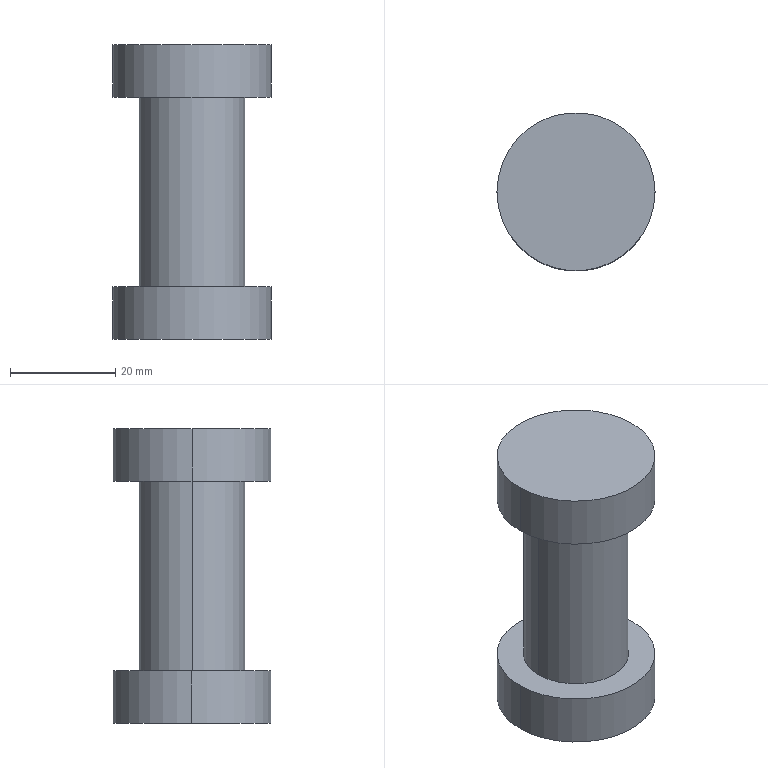Part | SolidWorks | features ICE 2, Extrusion 1 | 1 solid | 10 faces | box 30 x 30 x 56 mm | volume 25447 mm3 | cylinder 6 | plane 4 | commonest cylinder face diameters 30 x4 20 x2
STEP:
#1=CARTESIAN_POINT('',(-15.,0.,-10.));
#2=VERTEX_POINT('',#1);
#3=CARTESIAN_POINT('',(15.,0.,-10.));
#4=VERTEX_POINT('',#3);
#5=CARTESIAN_POINT('',(0.,0.,-10.));
#6=DIRECTION('',(0.,0.,-1.));
#7=DIRECTION('',(-1.,0.,0.));
#8=AXIS2_PLACEMENT_3D('',#5,#6,#7);
#9=CIRCLE('',#8,15.);
#10=EDGE_CURVE('',#2,#4,#9,.T.);
#11=ORIENTED_EDGE('',*,*,#10,.F.);
#12=CARTESIAN_POINT('',(-15.,0.,0.));
#13=VERTEX_POINT('',#12);
#14=CARTESIAN_POINT('',(-15.,0.,-10.));
#15=DIRECTION('',(0.,0.,1.));
#16=VECTOR('',#15,1000.);
#17=LINE('',#14,#16);
#18=EDGE_CURVE('',#2,#13,#17,.T.);
#19=ORIENTED_EDGE('',*,*,#18,.T.);
#20=CARTESIAN_POINT('',(15.,0.,0.));
#21=VERTEX_POINT('',#20);
#22=CARTESIAN_POINT('',(0.,0.,0.));
#23=DIRECTION('',(0.,0.,-1.));
#24=DIRECTION('',(-1.,0.,0.));
#25=AXIS2_PLACEMENT_3D('',#22,#23,#24);
#26=CIRCLE('',#25,15.);
#27=EDGE_CURVE('',#13,#21,#26,.T.);
#28=ORIENTED_EDGE('',*,*,#27,.T.);
#29=CARTESIAN_POINT('',(15.,0.,-10.));
#30=DIRECTION('',(0.,0.,1.));
#31=VECTOR('',#30,1000.);
#32=LINE('',#29,#31);
#33=EDGE_CURVE('',#4,#21,#32,.T.);
#34=ORIENTED_EDGE('',*,*,#33,.F.);
#35=EDGE_LOOP('',(#11,#19,#28,#34));
#36=FACE_OUTER_BOUND('',#35,.T.);
#37=CARTESIAN_POINT('',(0.,0.,-10.));
#38=DIRECTION('',(0.,0.,1.));
#39=DIRECTION('',(1.,0.,0.));
#40=AXIS2_PLACEMENT_3D('',#37,#38,#39);
#41=CYLINDRICAL_SURFACE('',#40,15.);
#42=ADVANCED_FACE('',(#36),#41,.T.);
#43=CARTESIAN_POINT('',(15.,0.,46.));
#44=VERTEX_POINT('',#43);
#45=CARTESIAN_POINT('',(-15.,0.,46.));
#46=VERTEX_POINT('',#45);
#47=CARTESIAN_POINT('',(0.,0.,46.));
#48=DIRECTION('',(0.,0.,1.));
#49=DIRECTION('',(1.,0.,0.));
#50=AXIS2_PLACEMENT_3D('',#47,#48,#49);
#51=CIRCLE('',#50,15.);
#52=EDGE_CURVE('',#44,#46,#51,.T.);
#53=ORIENTED_EDGE('',*,*,#52,.F.);
#54=CARTESIAN_POINT('',(15.,0.,36.));
#55=VERTEX_POINT('',#54);
#56=CARTESIAN_POINT('',(15.,0.,46.));
#57=DIRECTION('',(0.,0.,-1.));
#58=VECTOR('',#57,1000.);
#59=LINE('',#56,#58);
#60=EDGE_CURVE('',#44,#55,#59,.T.);
#61=ORIENTED_EDGE('',*,*,#60,.T.);
#62=CARTESIAN_POINT('',(-15.,0.,36.));
#63=VERTEX_POINT('',#62);
#64=CARTESIAN_POINT('',(0.,0.,36.));
#65=DIRECTION('',(0.,0.,1.));
#66=DIRECTION('',(1.,0.,0.));
#67=AXIS2_PLACEMENT_3D('',#64,#65,#66);
#68=CIRCLE('',#67,15.);
#69=EDGE_CURVE('',#55,#63,#68,.T.);
#70=ORIENTED_EDGE('',*,*,#69,.T.);
#71=CARTESIAN_POINT('',(-15.,0.,46.));
#72=DIRECTION('',(0.,0.,-1.));
#73=VECTOR('',#72,1000.);
#74=LINE('',#71,#73);
#75=EDGE_CURVE('',#46,#63,#74,.T.);
#76=ORIENTED_EDGE('',*,*,#75,.F.);
#77=EDGE_LOOP('',(#53,#61,#70,#76));
#78=FACE_OUTER_BOUND('',#77,.T.);
#79=CARTESIAN_POINT('',(0.,0.,46.));
#80=DIRECTION('',(0.,0.,-1.));
#81=DIRECTION('',(-1.,0.,0.));
#82=AXIS2_PLACEMENT_3D('',#79,#80,#81);
#83=CYLINDRICAL_SURFACE('',#82,15.);
#84=ADVANCED_FACE('',(#78),#83,.T.);
#85=CARTESIAN_POINT('',(10.,0.,36.));
#86=VERTEX_POINT('',#85);
#87=CARTESIAN_POINT('',(-10.,0.,36.));
#88=VERTEX_POINT('',#87);
#89=CARTESIAN_POINT('',(0.,0.,36.));
#90=DIRECTION('',(0.,0.,1.));
#91=DIRECTION('',(1.,0.,0.));
#92=AXIS2_PLACEMENT_3D('',#89,#90,#91);
#93=CIRCLE('',#92,10.);
#94=EDGE_CURVE('',#86,#88,#93,.T.);
#95=ORIENTED_EDGE('',*,*,#94,.F.);
#96=CARTESIAN_POINT('',(10.,0.,0.));
#97=VERTEX_POINT('',#96);
#98=CARTESIAN_POINT('',(10.,0.,36.));
#99=DIRECTION('',(0.,0.,-1.));
#100=VECTOR('',#99,1000.);
#101=LINE('',#98,#100);
#102=EDGE_CURVE('',#86,#97,#101,.T.);
#103=ORIENTED_EDGE('',*,*,#102,.T.);
#104=CARTESIAN_POINT('',(-10.,0.,0.));
#105=VERTEX_POINT('',#104);
#106=CARTESIAN_POINT('',(0.,0.,0.));
#107=DIRECTION('',(0.,0.,1.));
#108=DIRECTION('',(1.,0.,0.));
#109=AXIS2_PLACEMENT_3D('',#106,#107,#108);
#110=CIRCLE('',#109,10.);
#111=EDGE_CURVE('',#97,#105,#110,.T.);
#112=ORIENTED_EDGE('',*,*,#111,.T.);
#113=CARTESIAN_POINT('',(-10.,0.,36.));
#114=DIRECTION('',(0.,0.,-1.));
#115=VECTOR('',#114,1000.);
#116=LINE('',#113,#115);
#117=EDGE_CURVE('',#88,#105,#116,.T.);
#118=ORIENTED_EDGE('',*,*,#117,.F.);
#119=EDGE_LOOP('',(#95,#103,#112,#118));
#120=FACE_OUTER_BOUND('',#119,.T.);
#121=CARTESIAN_POINT('',(0.,0.,36.));
#122=DIRECTION('',(0.,0.,-1.));
#123=DIRECTION('',(-1.,0.,0.));
#124=AXIS2_PLACEMENT_3D('',#121,#122,#123);
#125=CYLINDRICAL_SURFACE('',#124,10.);
#126=ADVANCED_FACE('',(#120),#125,.T.);
#127=ORIENTED_EDGE('',*,*,#102,.F.);
#128=CARTESIAN_POINT('',(0.,0.,36.));
#129=DIRECTION('',(0.,0.,1.));
#130=DIRECTION('',(1.,0.,0.));
#131=AXIS2_PLACEMENT_3D('',#128,#129,#130);
#132=CIRCLE('',#131,10.);
#133=EDGE_CURVE('',#88,#86,#132,.T.);
#134=ORIENTED_EDGE('',*,*,#133,.F.);
#135=ORIENTED_EDGE('',*,*,#117,.T.);
#136=CARTESIAN_POINT('',(0.,0.,0.));
#137=DIRECTION('',(0.,0.,1.));
#138=DIRECTION('',(1.,0.,0.));
#139=AXIS2_PLACEMENT_3D('',#136,#137,#138);
#140=CIRCLE('',#139,10.);
#141=EDGE_CURVE('',#105,#97,#140,.T.);
#142=ORIENTED_EDGE('',*,*,#141,.T.);
#143=EDGE_LOOP('',(#127,#134,#135,#142));
#144=FACE_OUTER_BOUND('',#143,.T.);
#145=CARTESIAN_POINT('',(0.,0.,36.));
#146=DIRECTION('',(0.,0.,-1.));
#147=DIRECTION('',(-1.,0.,0.));
#148=AXIS2_PLACEMENT_3D('',#145,#146,#147);
#149=CYLINDRICAL_SURFACE('',#148,10.);
#150=ADVANCED_FACE('',(#144),#149,.T.);
#151=ORIENTED_EDGE('',*,*,#60,.F.);
#152=CARTESIAN_POINT('',(0.,0.,46.));
#153=DIRECTION('',(0.,0.,1.));
#154=DIRECTION('',(1.,0.,0.));
#155=AXIS2_PLACEMENT_3D('',#152,#153,#154);
#156=CIRCLE('',#155,15.);
#157=EDGE_CURVE('',#46,#44,#156,.T.);
#158=ORIENTED_EDGE('',*,*,#157,.F.);
#159=ORIENTED_EDGE('',*,*,#75,.T.);
#160=CARTESIAN_POINT('',(0.,0.,36.));
#161=DIRECTION('',(0.,0.,1.));
#162=DIRECTION('',(1.,0.,0.));
#163=AXIS2_PLACEMENT_3D('',#160,#161,#162);
#164=CIRCLE('',#163,15.);
#165=EDGE_CURVE('',#63,#55,#164,.T.);
#166=ORIENTED_EDGE('',*,*,#165,.T.);
#167=EDGE_LOOP('',(#151,#158,#159,#166));
#168=FACE_OUTER_BOUND('',#167,.T.);
#169=CARTESIAN_POINT('',(0.,0.,46.));
#170=DIRECTION('',(0.,0.,-1.));
#171=DIRECTION('',(-1.,0.,0.));
#172=AXIS2_PLACEMENT_3D('',#169,#170,#171);
#173=CYLINDRICAL_SURFACE('',#172,15.);
#174=ADVANCED_FACE('',(#168),#173,.T.);
#175=ORIENTED_EDGE('',*,*,#157,.T.);
#176=ORIENTED_EDGE('',*,*,#52,.T.);
#177=EDGE_LOOP('',(#175,#176));
#178=FACE_OUTER_BOUND('',#177,.T.);
#179=CARTESIAN_POINT('',(0.,0.,46.));
#180=DIRECTION('',(0.,0.,1.));
#181=DIRECTION('',(1.,0.,0.));
#182=AXIS2_PLACEMENT_3D('',#179,#180,#181);
#183=PLANE('',#182);
#184=ADVANCED_FACE('',(#178),#183,.T.);
#185=ORIENTED_EDGE('',*,*,#133,.T.);
#186=ORIENTED_EDGE('',*,*,#94,.T.);
#187=EDGE_LOOP('',(#185,#186));
#188=FACE_BOUND('',#187,.T.);
#189=ORIENTED_EDGE('',*,*,#165,.F.);
#190=ORIENTED_EDGE('',*,*,#69,.F.);
#191=EDGE_LOOP('',(#189,#190));
#192=FACE_OUTER_BOUND('',#191,.T.);
#193=CARTESIAN_POINT('',(0.,0.,36.));
#194=DIRECTION('',(0.,0.,1.));
#195=DIRECTION('',(1.,0.,0.));
#196=AXIS2_PLACEMENT_3D('',#193,#194,#195);
#197=PLANE('',#196);
#198=ADVANCED_FACE('',(#188,#192),#197,.F.);
#199=ORIENTED_EDGE('',*,*,#18,.F.);
#200=CARTESIAN_POINT('',(0.,0.,-10.));
#201=DIRECTION('',(0.,0.,-1.));
#202=DIRECTION('',(-1.,0.,0.));
#203=AXIS2_PLACEMENT_3D('',#200,#201,#202);
#204=CIRCLE('',#203,15.);
#205=EDGE_CURVE('',#4,#2,#204,.T.);
#206=ORIENTED_EDGE('',*,*,#205,.F.);
#207=ORIENTED_EDGE('',*,*,#33,.T.);
#208=CARTESIAN_POINT('',(0.,0.,0.));
#209=DIRECTION('',(0.,0.,-1.));
#210=DIRECTION('',(-1.,0.,0.));
#211=AXIS2_PLACEMENT_3D('',#208,#209,#210);
#212=CIRCLE('',#211,15.);
#213=EDGE_CURVE('',#21,#13,#212,.T.);
#214=ORIENTED_EDGE('',*,*,#213,.T.);
#215=EDGE_LOOP('',(#199,#206,#207,#214));
#216=FACE_OUTER_BOUND('',#215,.T.);
#217=CARTESIAN_POINT('',(0.,0.,-10.));
#218=DIRECTION('',(0.,0.,1.));
#219=DIRECTION('',(1.,0.,0.));
#220=AXIS2_PLACEMENT_3D('',#217,#218,#219);
#221=CYLINDRICAL_SURFACE('',#220,15.);
#222=ADVANCED_FACE('',(#216),#221,.T.);
#223=ORIENTED_EDGE('',*,*,#205,.T.);
#224=ORIENTED_EDGE('',*,*,#10,.T.);
#225=EDGE_LOOP('',(#223,#224));
#226=FACE_OUTER_BOUND('',#225,.T.);
#227=CARTESIAN_POINT('',(0.,0.,-10.));
#228=DIRECTION('',(0.,0.,-1.));
#229=DIRECTION('',(-1.,0.,0.));
#230=AXIS2_PLACEMENT_3D('',#227,#228,#229);
#231=PLANE('',#230);
#232=ADVANCED_FACE('',(#226),#231,.T.);
#233=ORIENTED_EDGE('',*,*,#141,.F.);
#234=ORIENTED_EDGE('',*,*,#111,.F.);
#235=EDGE_LOOP('',(#233,#234));
#236=FACE_BOUND('',#235,.T.);
#237=ORIENTED_EDGE('',*,*,#213,.F.);
#238=ORIENTED_EDGE('',*,*,#27,.F.);
#239=EDGE_LOOP('',(#237,#238));
#240=FACE_OUTER_BOUND('',#239,.T.);
#241=CARTESIAN_POINT('',(0.,0.,0.));
#242=DIRECTION('',(0.,0.,-1.));
#243=DIRECTION('',(-1.,0.,0.));
#244=AXIS2_PLACEMENT_3D('',#241,#242,#243);
#245=PLANE('',#244);
#246=ADVANCED_FACE('',(#236,#240),#245,.F.);
#247=CLOSED_SHELL('',(#42,#84,#126,#150,#174,#184,#198,#222,#232,#246));
#248=MANIFOLD_SOLID_BREP('',#247);
#249=CARTESIAN_POINT('',(0.,0.,0.));
#250=DIRECTION('',(0.,0.,1.));
#251=DIRECTION('',(1.,0.,0.));
#252=AXIS2_PLACEMENT_3D('',#249,#250,#251);
#253=(LENGTH_UNIT()NAMED_UNIT(*)SI_UNIT(.MILLI.,.METRE.));
#254=UNCERTAINTY_MEASURE_WITH_UNIT(LENGTH_MEASURE(0.00001),#253,'','');
#255=(NAMED_UNIT(*)PLANE_ANGLE_UNIT()SI_UNIT($,.RADIAN.));
#256=(NAMED_UNIT(*)SI_UNIT($,.STERADIAN.)SOLID_ANGLE_UNIT());
#257=(GEOMETRIC_REPRESENTATION_CONTEXT(3)GLOBAL_UNCERTAINTY_ASSIGNED_CONTEXT((#254))GLOBAL_UNIT_ASSIGNED_CONTEXT((#253,#255,#256))REPRESENTATION_CONTEXT('',''));
#258=ADVANCED_BREP_SHAPE_REPRESENTATION('',(#248,#252),#257);